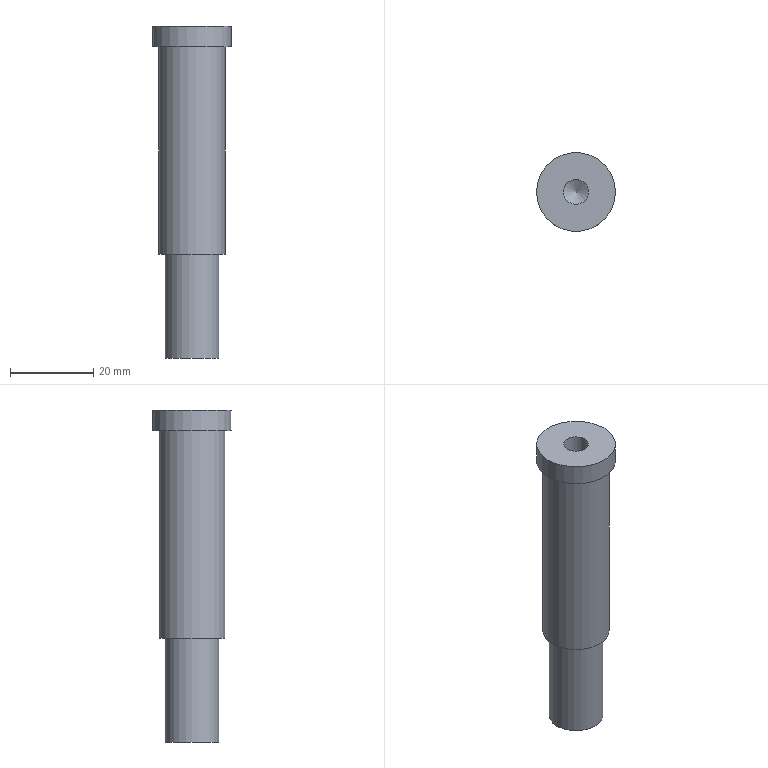Part | NX | features solid 2 | 1 solid | 9 faces | box 19 x 19 x 80 mm | volume 14405 mm3 | cylinder 4 | plane 4 | cone 1 | commonest cylinder face diameters 6 x1 13 x1 16 x1 19 x1
STEP:
#1=CARTESIAN_POINT('',(-170.,126.006,99.));
#2=VERTEX_POINT('',#1);
#3=CARTESIAN_POINT('',(-162.,126.006,99.));
#4=DIRECTION('',(0.,0.,1.));
#5=DIRECTION('',(-1.,0.,0.));
#6=AXIS2_PLACEMENT_3D('',#3,#4,#5);
#7=CIRCLE('',#6,8.);
#8=EDGE_CURVE('',#2,#2,#7,.T.);
#9=ORIENTED_EDGE('',*,*,#8,.T.);
#10=EDGE_LOOP('',(#9));
#11=FACE_BOUND('',#10,.T.);
#12=CARTESIAN_POINT('',(-170.,126.006,149.));
#13=VERTEX_POINT('',#12);
#14=CARTESIAN_POINT('',(-162.,126.006,149.));
#15=DIRECTION('',(0.,0.,1.));
#16=DIRECTION('',(-1.,0.,0.));
#17=AXIS2_PLACEMENT_3D('',#14,#15,#16);
#18=CIRCLE('',#17,8.);
#19=EDGE_CURVE('',#13,#13,#18,.T.);
#20=ORIENTED_EDGE('',*,*,#19,.F.);
#21=EDGE_LOOP('',(#20));
#22=FACE_BOUND('',#21,.T.);
#23=CARTESIAN_POINT('',(-162.,126.006,154.));
#24=DIRECTION('',(0.,0.,-1.));
#25=DIRECTION('',(1.,0.,0.));
#26=AXIS2_PLACEMENT_3D('',#23,#24,#25);
#27=CYLINDRICAL_SURFACE('',#26,8.);
#28=ADVANCED_FACE('',(#11,#22),#27,.T.);
#29=CARTESIAN_POINT('',(-168.5,126.006,99.));
#30=VERTEX_POINT('',#29);
#31=CARTESIAN_POINT('',(-162.,126.006,99.));
#32=DIRECTION('',(0.,0.,1.));
#33=DIRECTION('',(-1.,0.,0.));
#34=AXIS2_PLACEMENT_3D('',#31,#32,#33);
#35=CIRCLE('',#34,6.5);
#36=EDGE_CURVE('',#30,#30,#35,.T.);
#37=ORIENTED_EDGE('',*,*,#36,.T.);
#38=EDGE_LOOP('',(#37));
#39=FACE_BOUND('',#38,.T.);
#40=ORIENTED_EDGE('',*,*,#8,.F.);
#41=EDGE_LOOP('',(#40));
#42=FACE_BOUND('',#41,.T.);
#43=CARTESIAN_POINT('',(-162.,126.006,99.));
#44=DIRECTION('',(0.,0.,1.));
#45=DIRECTION('',(-1.,0.,0.));
#46=AXIS2_PLACEMENT_3D('',#43,#44,#45);
#47=PLANE('',#46);
#48=ADVANCED_FACE('',(#39,#42),#47,.F.);
#49=CARTESIAN_POINT('',(-171.5,126.006,149.));
#50=VERTEX_POINT('',#49);
#51=CARTESIAN_POINT('',(-162.,126.006,149.));
#52=DIRECTION('',(0.,0.,1.));
#53=DIRECTION('',(-1.,0.,0.));
#54=AXIS2_PLACEMENT_3D('',#51,#52,#53);
#55=CIRCLE('',#54,9.5);
#56=EDGE_CURVE('',#50,#50,#55,.T.);
#57=ORIENTED_EDGE('',*,*,#56,.F.);
#58=EDGE_LOOP('',(#57));
#59=FACE_BOUND('',#58,.T.);
#60=ORIENTED_EDGE('',*,*,#19,.T.);
#61=EDGE_LOOP('',(#60));
#62=FACE_BOUND('',#61,.T.);
#63=CARTESIAN_POINT('',(-162.,126.006,149.));
#64=DIRECTION('',(0.,0.,1.));
#65=DIRECTION('',(-1.,0.,0.));
#66=AXIS2_PLACEMENT_3D('',#63,#64,#65);
#67=PLANE('',#66);
#68=ADVANCED_FACE('',(#59,#62),#67,.F.);
#69=ORIENTED_EDGE('',*,*,#56,.T.);
#70=EDGE_LOOP('',(#69));
#71=FACE_BOUND('',#70,.T.);
#72=CARTESIAN_POINT('',(-171.5,126.006,154.));
#73=VERTEX_POINT('',#72);
#74=CARTESIAN_POINT('',(-162.,126.006,154.));
#75=DIRECTION('',(0.,0.,1.));
#76=DIRECTION('',(-1.,0.,0.));
#77=AXIS2_PLACEMENT_3D('',#74,#75,#76);
#78=CIRCLE('',#77,9.5);
#79=EDGE_CURVE('',#73,#73,#78,.T.);
#80=ORIENTED_EDGE('',*,*,#79,.F.);
#81=EDGE_LOOP('',(#80));
#82=FACE_BOUND('',#81,.T.);
#83=CARTESIAN_POINT('',(-162.,126.006,149.));
#84=DIRECTION('',(0.,0.,1.));
#85=DIRECTION('',(-1.,0.,0.));
#86=AXIS2_PLACEMENT_3D('',#83,#84,#85);
#87=CYLINDRICAL_SURFACE('',#86,9.5);
#88=ADVANCED_FACE('',(#71,#82),#87,.T.);
#89=CARTESIAN_POINT('',(-159.,126.006,154.));
#90=VERTEX_POINT('',#89);
#91=CARTESIAN_POINT('',(-162.,126.006,154.));
#92=DIRECTION('',(0.,0.,-1.));
#93=DIRECTION('',(1.,0.,0.));
#94=AXIS2_PLACEMENT_3D('',#91,#92,#93);
#95=CIRCLE('',#94,3.);
#96=EDGE_CURVE('',#90,#90,#95,.T.);
#97=ORIENTED_EDGE('',*,*,#96,.T.);
#98=EDGE_LOOP('',(#97));
#99=FACE_BOUND('',#98,.T.);
#100=ORIENTED_EDGE('',*,*,#79,.T.);
#101=EDGE_LOOP('',(#100));
#102=FACE_BOUND('',#101,.T.);
#103=CARTESIAN_POINT('',(-162.,126.006,154.));
#104=DIRECTION('',(0.,0.,1.));
#105=DIRECTION('',(-1.,0.,0.));
#106=AXIS2_PLACEMENT_3D('',#103,#104,#105);
#107=PLANE('',#106);
#108=ADVANCED_FACE('',(#99,#102),#107,.T.);
#109=CARTESIAN_POINT('',(-168.5,126.006,74.));
#110=VERTEX_POINT('',#109);
#111=CARTESIAN_POINT('',(-162.,126.006,74.));
#112=DIRECTION('',(0.,0.,1.));
#113=DIRECTION('',(-1.,0.,0.));
#114=AXIS2_PLACEMENT_3D('',#111,#112,#113);
#115=CIRCLE('',#114,6.5);
#116=EDGE_CURVE('',#110,#110,#115,.T.);
#117=ORIENTED_EDGE('',*,*,#116,.T.);
#118=EDGE_LOOP('',(#117));
#119=FACE_BOUND('',#118,.T.);
#120=ORIENTED_EDGE('',*,*,#36,.F.);
#121=EDGE_LOOP('',(#120));
#122=FACE_BOUND('',#121,.T.);
#123=CARTESIAN_POINT('',(-162.,126.006,74.));
#124=DIRECTION('',(0.,0.,1.));
#125=DIRECTION('',(-1.,0.,0.));
#126=AXIS2_PLACEMENT_3D('',#123,#124,#125);
#127=CYLINDRICAL_SURFACE('',#126,6.5);
#128=ADVANCED_FACE('',(#119,#122),#127,.T.);
#129=ORIENTED_EDGE('',*,*,#116,.F.);
#130=EDGE_LOOP('',(#129));
#131=FACE_BOUND('',#130,.T.);
#132=CARTESIAN_POINT('',(-162.,126.006,74.));
#133=DIRECTION('',(0.,0.,1.));
#134=DIRECTION('',(-1.,0.,0.));
#135=AXIS2_PLACEMENT_3D('',#132,#133,#134);
#136=PLANE('',#135);
#137=ADVANCED_FACE('',(#131),#136,.F.);
#138=CARTESIAN_POINT('',(-159.,126.006,141.));
#139=VERTEX_POINT('',#138);
#140=CARTESIAN_POINT('',(-162.,126.006,141.));
#141=DIRECTION('',(0.,0.,-1.));
#142=DIRECTION('',(1.,0.,0.));
#143=AXIS2_PLACEMENT_3D('',#140,#141,#142);
#144=CIRCLE('',#143,3.);
#145=EDGE_CURVE('',#139,#139,#144,.T.);
#146=ORIENTED_EDGE('',*,*,#145,.F.);
#147=EDGE_LOOP('',(#146));
#148=FACE_BOUND('',#147,.T.);
#149=CARTESIAN_POINT('',(-162.,126.006,139.268));
#150=VERTEX_POINT('',#149);
#151=VERTEX_LOOP('',#150);
#152=FACE_BOUND('',#151,.T.);
#153=CARTESIAN_POINT('',(-162.,126.006,141.));
#154=DIRECTION('',(0.,0.,1.));
#155=DIRECTION('',(-1.,0.,0.));
#156=AXIS2_PLACEMENT_3D('',#153,#154,#155);
#157=CONICAL_SURFACE('',#156,3.,1.047);
#158=ADVANCED_FACE('',(#148,#152),#157,.F.);
#159=ORIENTED_EDGE('',*,*,#145,.T.);
#160=EDGE_LOOP('',(#159));
#161=FACE_BOUND('',#160,.T.);
#162=ORIENTED_EDGE('',*,*,#96,.F.);
#163=EDGE_LOOP('',(#162));
#164=FACE_BOUND('',#163,.T.);
#165=CARTESIAN_POINT('',(-162.,126.006,154.));
#166=DIRECTION('',(0.,0.,-1.));
#167=DIRECTION('',(1.,0.,0.));
#168=AXIS2_PLACEMENT_3D('',#165,#166,#167);
#169=CYLINDRICAL_SURFACE('',#168,3.);
#170=ADVANCED_FACE('',(#161,#164),#169,.F.);
#171=CLOSED_SHELL('',(#28,#48,#68,#88,#108,#128,#137,#158,#170));
#172=MANIFOLD_SOLID_BREP('',#171);
#173=(LENGTH_UNIT()NAMED_UNIT(*)SI_UNIT(.MILLI.,.METRE.));
#174=UNCERTAINTY_MEASURE_WITH_UNIT(LENGTH_MEASURE(0.00001),#173,'','');
#175=(NAMED_UNIT(*)PLANE_ANGLE_UNIT()SI_UNIT($,.RADIAN.));
#176=(NAMED_UNIT(*)SI_UNIT($,.STERADIAN.)SOLID_ANGLE_UNIT());
#177=(GEOMETRIC_REPRESENTATION_CONTEXT(3)GLOBAL_UNCERTAINTY_ASSIGNED_CONTEXT((#174))GLOBAL_UNIT_ASSIGNED_CONTEXT((#173,#175,#176))REPRESENTATION_CONTEXT('',''));
#178=ADVANCED_BREP_SHAPE_REPRESENTATION('',(#172),#177);